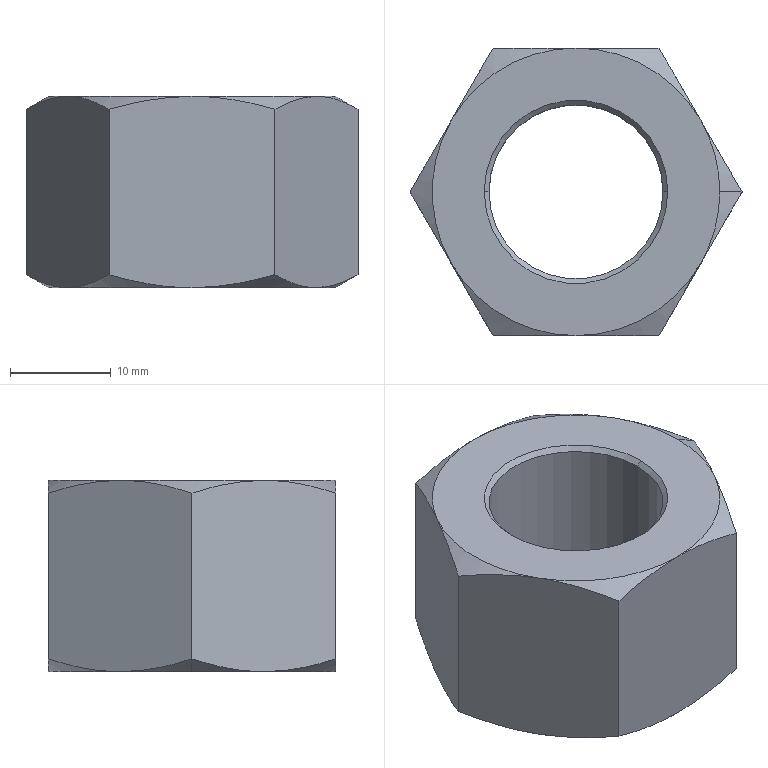Part | SolidWorks | 1 solid | 28 faces | box 33 x 28.579 x 19 mm | volume 8913 mm3 | cone 18 | plane 8 | cylinder 2 | commonest cylinder face diameters 17.294 x2
STEP:
#1=CARTESIAN_POINT('',(-8.647,0.,18.525));
#2=VERTEX_POINT('',#1);
#3=CARTESIAN_POINT('',(8.647,0.,18.525));
#4=VERTEX_POINT('',#3);
#5=CARTESIAN_POINT('',(0.,0.,18.525));
#6=DIRECTION('',(0.,0.,1.));
#7=DIRECTION('',(1.,0.,0.));
#8=AXIS2_PLACEMENT_3D('',#5,#6,#7);
#9=CIRCLE('',#8,8.647);
#10=EDGE_CURVE('',#2,#4,#9,.T.);
#11=ORIENTED_EDGE('',*,*,#10,.F.);
#12=CARTESIAN_POINT('',(-9.122,0.,19.));
#13=VERTEX_POINT('',#12);
#14=CARTESIAN_POINT('',(-8.647,0.,18.525));
#15=DIRECTION('',(-0.7071,0.,0.7071));
#16=VECTOR('',#15,1000.);
#17=LINE('',#14,#16);
#18=EDGE_CURVE('',#2,#13,#17,.T.);
#19=ORIENTED_EDGE('',*,*,#18,.T.);
#20=CARTESIAN_POINT('',(9.122,0.,19.));
#21=VERTEX_POINT('',#20);
#22=CARTESIAN_POINT('',(0.,0.,19.));
#23=DIRECTION('',(0.,0.,-1.));
#24=DIRECTION('',(1.,0.,0.));
#25=AXIS2_PLACEMENT_3D('',#22,#23,#24);
#26=CIRCLE('',#25,9.122);
#27=EDGE_CURVE('',#21,#13,#26,.T.);
#28=ORIENTED_EDGE('',*,*,#27,.F.);
#29=CARTESIAN_POINT('',(8.647,0.,18.525));
#30=DIRECTION('',(0.7071,0.,0.7071));
#31=VECTOR('',#30,1000.);
#32=LINE('',#29,#31);
#33=EDGE_CURVE('',#4,#21,#32,.T.);
#34=ORIENTED_EDGE('',*,*,#33,.F.);
#35=EDGE_LOOP('',(#11,#19,#28,#34));
#36=FACE_OUTER_BOUND('',#35,.T.);
#37=CARTESIAN_POINT('',(0.,0.,18.525));
#38=DIRECTION('',(0.,0.,1.));
#39=DIRECTION('',(1.,0.,0.));
#40=AXIS2_PLACEMENT_3D('',#37,#38,#39);
#41=CONICAL_SURFACE('',#40,8.647,0.7854);
#42=ADVANCED_FACE('',(#36),#41,.F.);
#43=CARTESIAN_POINT('',(8.647,0.,0.475));
#44=VERTEX_POINT('',#43);
#45=CARTESIAN_POINT('',(-8.647,0.,0.475));
#46=VERTEX_POINT('',#45);
#47=CARTESIAN_POINT('',(0.,0.,0.475));
#48=DIRECTION('',(0.,0.,-1.));
#49=DIRECTION('',(1.,0.,0.));
#50=AXIS2_PLACEMENT_3D('',#47,#48,#49);
#51=CIRCLE('',#50,8.647);
#52=EDGE_CURVE('',#44,#46,#51,.T.);
#53=ORIENTED_EDGE('',*,*,#52,.F.);
#54=CARTESIAN_POINT('',(9.122,0.,0.));
#55=VERTEX_POINT('',#54);
#56=CARTESIAN_POINT('',(9.122,0.,0.));
#57=DIRECTION('',(0.7071,0.,-0.7071));
#58=VECTOR('',#57,1000.);
#59=LINE('',#56,#58);
#60=EDGE_CURVE('',#44,#55,#59,.T.);
#61=ORIENTED_EDGE('',*,*,#60,.T.);
#62=CARTESIAN_POINT('',(-9.122,0.,0.));
#63=VERTEX_POINT('',#62);
#64=CARTESIAN_POINT('',(0.,0.,0.));
#65=DIRECTION('',(0.,0.,1.));
#66=DIRECTION('',(1.,0.,0.));
#67=AXIS2_PLACEMENT_3D('',#64,#65,#66);
#68=CIRCLE('',#67,9.122);
#69=EDGE_CURVE('',#63,#55,#68,.T.);
#70=ORIENTED_EDGE('',*,*,#69,.F.);
#71=CARTESIAN_POINT('',(-9.122,0.,0.));
#72=DIRECTION('',(-0.7071,0.,-0.7071));
#73=VECTOR('',#72,1000.);
#74=LINE('',#71,#73);
#75=EDGE_CURVE('',#46,#63,#74,.T.);
#76=ORIENTED_EDGE('',*,*,#75,.F.);
#77=EDGE_LOOP('',(#53,#61,#70,#76));
#78=FACE_OUTER_BOUND('',#77,.T.);
#79=CARTESIAN_POINT('',(0.,0.,0.));
#80=DIRECTION('',(0.,0.,-1.));
#81=DIRECTION('',(-1.,0.,0.));
#82=AXIS2_PLACEMENT_3D('',#79,#80,#81);
#83=CONICAL_SURFACE('',#82,9.122,0.7854);
#84=ADVANCED_FACE('',(#78),#83,.F.);
#85=CARTESIAN_POINT('',(14.289,0.,19.));
#86=VERTEX_POINT('',#85);
#87=CARTESIAN_POINT('',(12.375,7.145,19.));
#88=VERTEX_POINT('',#87);
#89=CARTESIAN_POINT('',(0.,0.,19.));
#90=DIRECTION('',(0.,0.,1.));
#91=DIRECTION('',(1.,0.,0.));
#92=AXIS2_PLACEMENT_3D('',#89,#90,#91);
#93=CIRCLE('',#92,14.289);
#94=EDGE_CURVE('',#86,#88,#93,.T.);
#95=ORIENTED_EDGE('',*,*,#94,.F.);
#96=CARTESIAN_POINT('',(16.5,0.,17.724));
#97=VERTEX_POINT('',#96);
#98=CARTESIAN_POINT('',(14.289,0.,19.));
#99=DIRECTION('',(0.866,0.,-0.5));
#100=VECTOR('',#99,1000.);
#101=LINE('',#98,#100);
#102=EDGE_CURVE('',#86,#97,#101,.T.);
#103=ORIENTED_EDGE('',*,*,#102,.T.);
#104=CARTESIAN_POINT('',(16.5,0.,17.724));
#105=CARTESIAN_POINT('',(15.825,1.169,18.113));
#106=CARTESIAN_POINT('',(15.145,2.346,18.434));
#107=CARTESIAN_POINT('',(13.772,4.725,18.878));
#108=CARTESIAN_POINT('',(13.078,5.927,19.));
#109=CARTESIAN_POINT('',(12.375,7.145,19.));
#110=B_SPLINE_CURVE_WITH_KNOTS('',3,(#104,#105,#106,#107,#108,#109),.UNSPECIFIED.,.F.,.F.,(4,2,4),(0.000000238,0.004174,0.008348),.UNSPECIFIED.);
#111=EDGE_CURVE('',#97,#88,#110,.T.);
#112=ORIENTED_EDGE('',*,*,#111,.T.);
#113=EDGE_LOOP('',(#95,#103,#112));
#114=FACE_OUTER_BOUND('',#113,.T.);
#115=CARTESIAN_POINT('',(0.,0.,19.));
#116=DIRECTION('',(0.,0.,-1.));
#117=DIRECTION('',(1.,0.,0.));
#118=AXIS2_PLACEMENT_3D('',#115,#116,#117);
#119=CONICAL_SURFACE('',#118,14.289,1.047);
#120=ADVANCED_FACE('',(#114),#119,.T.);
#121=CARTESIAN_POINT('',(-14.289,0.,0.));
#122=VERTEX_POINT('',#121);
#123=CARTESIAN_POINT('',(-12.375,7.145,0.));
#124=VERTEX_POINT('',#123);
#125=CARTESIAN_POINT('',(0.,0.,0.));
#126=DIRECTION('',(0.,0.,-1.));
#127=DIRECTION('',(-1.,0.,0.));
#128=AXIS2_PLACEMENT_3D('',#125,#126,#127);
#129=CIRCLE('',#128,14.289);
#130=EDGE_CURVE('',#122,#124,#129,.T.);
#131=ORIENTED_EDGE('',*,*,#130,.F.);
#132=CARTESIAN_POINT('',(-16.5,0.,1.276));
#133=VERTEX_POINT('',#132);
#134=CARTESIAN_POINT('',(-14.289,0.,0.));
#135=DIRECTION('',(-0.866,0.,0.5));
#136=VECTOR('',#135,1000.);
#137=LINE('',#134,#136);
#138=EDGE_CURVE('',#122,#133,#137,.T.);
#139=ORIENTED_EDGE('',*,*,#138,.T.);
#140=CARTESIAN_POINT('',(-16.5,0.,1.276));
#141=CARTESIAN_POINT('',(-15.825,1.169,0.8867));
#142=CARTESIAN_POINT('',(-15.145,2.346,0.5657));
#143=CARTESIAN_POINT('',(-13.772,4.725,0.1216));
#144=CARTESIAN_POINT('',(-13.078,5.927,0.));
#145=CARTESIAN_POINT('',(-12.375,7.145,0.));
#146=B_SPLINE_CURVE_WITH_KNOTS('',3,(#140,#141,#142,#143,#144,#145),.UNSPECIFIED.,.F.,.F.,(4,2,4),(0.000000238,0.004174,0.008348),.UNSPECIFIED.);
#147=EDGE_CURVE('',#133,#124,#146,.T.);
#148=ORIENTED_EDGE('',*,*,#147,.T.);
#149=EDGE_LOOP('',(#131,#139,#148));
#150=FACE_OUTER_BOUND('',#149,.T.);
#151=CARTESIAN_POINT('',(0.,0.,0.));
#152=DIRECTION('',(0.,0.,1.));
#153=DIRECTION('',(-1.,0.,0.));
#154=AXIS2_PLACEMENT_3D('',#151,#152,#153);
#155=CONICAL_SURFACE('',#154,14.289,1.047);
#156=ADVANCED_FACE('',(#150),#155,.T.);
#157=ORIENTED_EDGE('',*,*,#10,.T.);
#158=CARTESIAN_POINT('',(8.647,0.,19.));
#159=DIRECTION('',(0.,0.,-1.));
#160=VECTOR('',#159,1000.);
#161=LINE('',#158,#160);
#162=EDGE_CURVE('',#4,#44,#161,.T.);
#163=ORIENTED_EDGE('',*,*,#162,.T.);
#164=ORIENTED_EDGE('',*,*,#52,.T.);
#165=CARTESIAN_POINT('',(-8.647,0.,19.));
#166=DIRECTION('',(0.,0.,-1.));
#167=VECTOR('',#166,1000.);
#168=LINE('',#165,#167);
#169=EDGE_CURVE('',#2,#46,#168,.T.);
#170=ORIENTED_EDGE('',*,*,#169,.F.);
#171=EDGE_LOOP('',(#157,#163,#164,#170));
#172=FACE_OUTER_BOUND('',#171,.T.);
#173=CARTESIAN_POINT('',(0.,0.,19.));
#174=DIRECTION('',(0.,0.,-1.));
#175=DIRECTION('',(-1.,0.,0.));
#176=AXIS2_PLACEMENT_3D('',#173,#174,#175);
#177=CYLINDRICAL_SURFACE('',#176,8.647);
#178=ADVANCED_FACE('',(#172),#177,.F.);
#179=ORIENTED_EDGE('',*,*,#111,.F.);
#180=CARTESIAN_POINT('',(16.5,0.,1.276));
#181=VERTEX_POINT('',#180);
#182=CARTESIAN_POINT('',(16.5,0.,19.));
#183=DIRECTION('',(0.,0.,-1.));
#184=VECTOR('',#183,1000.);
#185=LINE('',#182,#184);
#186=EDGE_CURVE('',#97,#181,#185,.T.);
#187=ORIENTED_EDGE('',*,*,#186,.T.);
#188=CARTESIAN_POINT('',(12.375,7.145,0.));
#189=VERTEX_POINT('',#188);
#190=CARTESIAN_POINT('',(12.375,7.145,0.));
#191=CARTESIAN_POINT('',(12.725,6.538,0.));
#192=CARTESIAN_POINT('',(13.077,5.929,0.03017));
#193=CARTESIAN_POINT('',(13.772,4.724,0.1469));
#194=CARTESIAN_POINT('',(14.118,4.126,0.2334));
#195=CARTESIAN_POINT('',(15.148,2.341,0.5668));
#196=CARTESIAN_POINT('',(15.827,1.166,0.8877));
#197=CARTESIAN_POINT('',(16.5,0.,1.276));
#198=B_SPLINE_CURVE_WITH_KNOTS('',3,(#190,#191,#192,#193,#194,#195,#196,#197),.UNSPECIFIED.,.F.,.F.,(4,2,2,4),(0.008348,0.01043,0.01251,0.01666),.UNSPECIFIED.);
#199=EDGE_CURVE('',#189,#181,#198,.T.);
#200=ORIENTED_EDGE('',*,*,#199,.F.);
#201=CARTESIAN_POINT('',(8.25,14.289,1.276));
#202=VERTEX_POINT('',#201);
#203=CARTESIAN_POINT('',(8.25,14.289,1.276));
#204=CARTESIAN_POINT('',(8.925,13.121,0.8867));
#205=CARTESIAN_POINT('',(9.605,11.943,0.5657));
#206=CARTESIAN_POINT('',(10.978,9.564,0.1216));
#207=CARTESIAN_POINT('',(11.672,8.362,0.));
#208=CARTESIAN_POINT('',(12.375,7.145,0.));
#209=B_SPLINE_CURVE_WITH_KNOTS('',3,(#203,#204,#205,#206,#207,#208),.UNSPECIFIED.,.F.,.F.,(4,2,4),(0.000000238,0.004174,0.008348),.UNSPECIFIED.);
#210=EDGE_CURVE('',#202,#189,#209,.T.);
#211=ORIENTED_EDGE('',*,*,#210,.F.);
#212=CARTESIAN_POINT('',(8.25,14.289,17.724));
#213=VERTEX_POINT('',#212);
#214=CARTESIAN_POINT('',(8.25,14.289,19.));
#215=DIRECTION('',(0.,0.,-1.));
#216=VECTOR('',#215,1000.);
#217=LINE('',#214,#216);
#218=EDGE_CURVE('',#213,#202,#217,.T.);
#219=ORIENTED_EDGE('',*,*,#218,.F.);
#220=CARTESIAN_POINT('',(12.375,7.145,19.));
#221=CARTESIAN_POINT('',(12.025,7.751,19.));
#222=CARTESIAN_POINT('',(11.673,8.36,18.97));
#223=CARTESIAN_POINT('',(10.978,9.565,18.853));
#224=CARTESIAN_POINT('',(10.632,10.163,18.767));
#225=CARTESIAN_POINT('',(9.602,11.948,18.433));
#226=CARTESIAN_POINT('',(8.923,13.124,18.112));
#227=CARTESIAN_POINT('',(8.25,14.289,17.724));
#228=B_SPLINE_CURVE_WITH_KNOTS('',3,(#220,#221,#222,#223,#224,#225,#226,#227),.UNSPECIFIED.,.F.,.F.,(4,2,2,4),(0.008348,0.01043,0.01251,0.01666),.UNSPECIFIED.);
#229=EDGE_CURVE('',#88,#213,#228,.T.);
#230=ORIENTED_EDGE('',*,*,#229,.F.);
#231=EDGE_LOOP('',(#179,#187,#200,#211,#219,#230));
#232=FACE_OUTER_BOUND('',#231,.T.);
#233=CARTESIAN_POINT('',(16.5,0.,19.));
#234=DIRECTION('',(-0.866,-0.5,0.));
#235=DIRECTION('',(0.5,-0.866,0.));
#236=AXIS2_PLACEMENT_3D('',#233,#234,#235);
#237=PLANE('',#236);
#238=ADVANCED_FACE('',(#232),#237,.F.);
#239=CARTESIAN_POINT('',(0.,14.289,19.));
#240=VERTEX_POINT('',#239);
#241=CARTESIAN_POINT('',(8.25,14.289,17.724));
#242=CARTESIAN_POINT('',(6.916,14.289,18.109));
#243=CARTESIAN_POINT('',(5.564,14.289,18.429));
#244=CARTESIAN_POINT('',(3.499,14.289,18.765));
#245=CARTESIAN_POINT('',(2.804,14.289,18.852));
#246=CARTESIAN_POINT('',(1.4,14.289,18.97));
#247=CARTESIAN_POINT('',(0.6982,14.289,19.));
#248=CARTESIAN_POINT('',(0.,14.289,19.));
#249=B_SPLINE_CURVE_WITH_KNOTS('',3,(#241,#242,#243,#244,#245,#246,#247,#248),.UNSPECIFIED.,.F.,.F.,(4,2,2,4),(0.04793,0.0521,0.05419,0.05628),.UNSPECIFIED.);
#250=EDGE_CURVE('',#213,#240,#249,.T.);
#251=ORIENTED_EDGE('',*,*,#250,.F.);
#252=ORIENTED_EDGE('',*,*,#218,.T.);
#253=CARTESIAN_POINT('',(0.,14.289,0.));
#254=VERTEX_POINT('',#253);
#255=CARTESIAN_POINT('',(0.,14.289,0.));
#256=CARTESIAN_POINT('',(0.6982,14.289,0.));
#257=CARTESIAN_POINT('',(1.4,14.289,0.02979));
#258=CARTESIAN_POINT('',(2.804,14.289,0.1478));
#259=CARTESIAN_POINT('',(3.499,14.289,0.2352));
#260=CARTESIAN_POINT('',(5.564,14.289,0.5705));
#261=CARTESIAN_POINT('',(6.916,14.289,0.8911));
#262=CARTESIAN_POINT('',(8.25,14.289,1.276));
#263=B_SPLINE_CURVE_WITH_KNOTS('',3,(#255,#256,#257,#258,#259,#260,#261,#262),.UNSPECIFIED.,.F.,.F.,(4,2,2,4),(0.02351,0.0256,0.02769,0.03187),.UNSPECIFIED.);
#264=EDGE_CURVE('',#254,#202,#263,.T.);
#265=ORIENTED_EDGE('',*,*,#264,.F.);
#266=CARTESIAN_POINT('',(-8.25,14.289,1.276));
#267=VERTEX_POINT('',#266);
#268=CARTESIAN_POINT('',(-8.25,14.289,1.276));
#269=CARTESIAN_POINT('',(-6.907,14.289,0.8886));
#270=CARTESIAN_POINT('',(-5.533,14.289,0.564));
#271=CARTESIAN_POINT('',(-2.781,14.289,0.12));
#272=CARTESIAN_POINT('',(-1.395,14.289,0.));
#273=CARTESIAN_POINT('',(0.,14.289,0.));
#274=B_SPLINE_CURVE_WITH_KNOTS('',3,(#268,#269,#270,#271,#272,#273),.UNSPECIFIED.,.F.,.F.,(4,2,4),(0.01516,0.01934,0.02351),.UNSPECIFIED.);
#275=EDGE_CURVE('',#267,#254,#274,.T.);
#276=ORIENTED_EDGE('',*,*,#275,.F.);
#277=CARTESIAN_POINT('',(-8.25,14.289,17.724));
#278=VERTEX_POINT('',#277);
#279=CARTESIAN_POINT('',(-8.25,14.289,19.));
#280=DIRECTION('',(0.,0.,-1.));
#281=VECTOR('',#280,1000.);
#282=LINE('',#279,#281);
#283=EDGE_CURVE('',#278,#267,#282,.T.);
#284=ORIENTED_EDGE('',*,*,#283,.F.);
#285=CARTESIAN_POINT('',(0.,14.289,19.));
#286=CARTESIAN_POINT('',(-1.395,14.289,19.));
#287=CARTESIAN_POINT('',(-2.781,14.289,18.88));
#288=CARTESIAN_POINT('',(-5.533,14.289,18.436));
#289=CARTESIAN_POINT('',(-6.907,14.289,18.111));
#290=CARTESIAN_POINT('',(-8.25,14.289,17.724));
#291=B_SPLINE_CURVE_WITH_KNOTS('',3,(#285,#286,#287,#288,#289,#290),.UNSPECIFIED.,.F.,.F.,(4,2,4),(0.05628,0.06045,0.06463),.UNSPECIFIED.);
#292=EDGE_CURVE('',#240,#278,#291,.T.);
#293=ORIENTED_EDGE('',*,*,#292,.F.);
#294=EDGE_LOOP('',(#251,#252,#265,#276,#284,#293));
#295=FACE_OUTER_BOUND('',#294,.T.);
#296=CARTESIAN_POINT('',(8.25,14.289,19.));
#297=DIRECTION('',(0.,-1.,0.));
#298=DIRECTION('',(1.,0.,0.));
#299=AXIS2_PLACEMENT_3D('',#296,#297,#298);
#300=PLANE('',#299);
#301=ADVANCED_FACE('',(#295),#300,.F.);
#302=CARTESIAN_POINT('',(-12.375,7.145,19.));
#303=VERTEX_POINT('',#302);
#304=CARTESIAN_POINT('',(-8.25,14.289,17.724));
#305=CARTESIAN_POINT('',(-8.925,13.121,18.113));
#306=CARTESIAN_POINT('',(-9.605,11.943,18.434));
#307=CARTESIAN_POINT('',(-10.978,9.564,18.878));
#308=CARTESIAN_POINT('',(-11.672,8.362,19.));
#309=CARTESIAN_POINT('',(-12.375,7.145,19.));
#310=B_SPLINE_CURVE_WITH_KNOTS('',3,(#304,#305,#306,#307,#308,#309),.UNSPECIFIED.,.F.,.F.,(4,2,4),(0.000000238,0.004174,0.008348),.UNSPECIFIED.);
#311=EDGE_CURVE('',#278,#303,#310,.T.);
#312=ORIENTED_EDGE('',*,*,#311,.F.);
#313=ORIENTED_EDGE('',*,*,#283,.T.);
#314=CARTESIAN_POINT('',(-12.375,7.145,0.));
#315=CARTESIAN_POINT('',(-12.025,7.751,0.));
#316=CARTESIAN_POINT('',(-11.673,8.36,0.03017));
#317=CARTESIAN_POINT('',(-10.978,9.565,0.1469));
#318=CARTESIAN_POINT('',(-10.632,10.163,0.2334));
#319=CARTESIAN_POINT('',(-9.602,11.948,0.5668));
#320=CARTESIAN_POINT('',(-8.923,13.124,0.8877));
#321=CARTESIAN_POINT('',(-8.25,14.289,1.276));
#322=B_SPLINE_CURVE_WITH_KNOTS('',3,(#314,#315,#316,#317,#318,#319,#320,#321),.UNSPECIFIED.,.F.,.F.,(4,2,2,4),(0.008348,0.01043,0.01251,0.01666),.UNSPECIFIED.);
#323=EDGE_CURVE('',#124,#267,#322,.T.);
#324=ORIENTED_EDGE('',*,*,#323,.F.);
#325=ORIENTED_EDGE('',*,*,#147,.F.);
#326=CARTESIAN_POINT('',(-16.5,0.,17.724));
#327=VERTEX_POINT('',#326);
#328=CARTESIAN_POINT('',(-16.5,0.,19.));
#329=DIRECTION('',(0.,0.,-1.));
#330=VECTOR('',#329,1000.);
#331=LINE('',#328,#330);
#332=EDGE_CURVE('',#327,#133,#331,.T.);
#333=ORIENTED_EDGE('',*,*,#332,.F.);
#334=CARTESIAN_POINT('',(-12.375,7.145,19.));
#335=CARTESIAN_POINT('',(-12.725,6.538,19.));
#336=CARTESIAN_POINT('',(-13.077,5.929,18.97));
#337=CARTESIAN_POINT('',(-13.772,4.724,18.853));
#338=CARTESIAN_POINT('',(-14.118,4.126,18.767));
#339=CARTESIAN_POINT('',(-15.148,2.341,18.433));
#340=CARTESIAN_POINT('',(-15.827,1.166,18.112));
#341=CARTESIAN_POINT('',(-16.5,0.,17.724));
#342=B_SPLINE_CURVE_WITH_KNOTS('',3,(#334,#335,#336,#337,#338,#339,#340,#341),.UNSPECIFIED.,.F.,.F.,(4,2,2,4),(0.008348,0.01043,0.01251,0.01666),.UNSPECIFIED.);
#343=EDGE_CURVE('',#303,#327,#342,.T.);
#344=ORIENTED_EDGE('',*,*,#343,.F.);
#345=EDGE_LOOP('',(#312,#313,#324,#325,#333,#344));
#346=FACE_OUTER_BOUND('',#345,.T.);
#347=CARTESIAN_POINT('',(-8.25,14.289,19.));
#348=DIRECTION('',(0.866,-0.5,0.));
#349=DIRECTION('',(0.5,0.866,0.));
#350=AXIS2_PLACEMENT_3D('',#347,#348,#349);
#351=PLANE('',#350);
#352=ADVANCED_FACE('',(#346),#351,.F.);
#353=CARTESIAN_POINT('',(-12.375,-7.145,19.));
#354=VERTEX_POINT('',#353);
#355=CARTESIAN_POINT('',(-16.5,0.,17.724));
#356=CARTESIAN_POINT('',(-15.825,-1.169,18.113));
#357=CARTESIAN_POINT('',(-15.145,-2.346,18.434));
#358=CARTESIAN_POINT('',(-13.772,-4.725,18.878));
#359=CARTESIAN_POINT('',(-13.078,-5.927,19.));
#360=CARTESIAN_POINT('',(-12.375,-7.145,19.));
#361=B_SPLINE_CURVE_WITH_KNOTS('',3,(#355,#356,#357,#358,#359,#360),.UNSPECIFIED.,.F.,.F.,(4,2,4),(0.000000238,0.004174,0.008348),.UNSPECIFIED.);
#362=EDGE_CURVE('',#327,#354,#361,.T.);
#363=ORIENTED_EDGE('',*,*,#362,.F.);
#364=ORIENTED_EDGE('',*,*,#332,.T.);
#365=CARTESIAN_POINT('',(-12.375,-7.145,0.));
#366=VERTEX_POINT('',#365);
#367=CARTESIAN_POINT('',(-12.375,-7.145,0.));
#368=CARTESIAN_POINT('',(-12.725,-6.538,0.));
#369=CARTESIAN_POINT('',(-13.077,-5.929,0.03017));
#370=CARTESIAN_POINT('',(-13.772,-4.724,0.1469));
#371=CARTESIAN_POINT('',(-14.118,-4.126,0.2334));
#372=CARTESIAN_POINT('',(-15.148,-2.341,0.5668));
#373=CARTESIAN_POINT('',(-15.827,-1.166,0.8877));
#374=CARTESIAN_POINT('',(-16.5,0.,1.276));
#375=B_SPLINE_CURVE_WITH_KNOTS('',3,(#367,#368,#369,#370,#371,#372,#373,#374),.UNSPECIFIED.,.F.,.F.,(4,2,2,4),(0.008348,0.01043,0.01251,0.01666),.UNSPECIFIED.);
#376=EDGE_CURVE('',#366,#133,#375,.T.);
#377=ORIENTED_EDGE('',*,*,#376,.F.);
#378=CARTESIAN_POINT('',(-8.25,-14.289,1.276));
#379=VERTEX_POINT('',#378);
#380=CARTESIAN_POINT('',(-8.25,-14.289,1.276));
#381=CARTESIAN_POINT('',(-8.925,-13.121,0.8867));
#382=CARTESIAN_POINT('',(-9.605,-11.943,0.5657));
#383=CARTESIAN_POINT('',(-10.978,-9.564,0.1216));
#384=CARTESIAN_POINT('',(-11.672,-8.362,0.));
#385=CARTESIAN_POINT('',(-12.375,-7.145,0.));
#386=B_SPLINE_CURVE_WITH_KNOTS('',3,(#380,#381,#382,#383,#384,#385),.UNSPECIFIED.,.F.,.F.,(4,2,4),(0.000000238,0.004174,0.008348),.UNSPECIFIED.);
#387=EDGE_CURVE('',#379,#366,#386,.T.);
#388=ORIENTED_EDGE('',*,*,#387,.F.);
#389=CARTESIAN_POINT('',(-8.25,-14.289,17.724));
#390=VERTEX_POINT('',#389);
#391=CARTESIAN_POINT('',(-8.25,-14.289,19.));
#392=DIRECTION('',(0.,0.,-1.));
#393=VECTOR('',#392,1000.);
#394=LINE('',#391,#393);
#395=EDGE_CURVE('',#390,#379,#394,.T.);
#396=ORIENTED_EDGE('',*,*,#395,.F.);
#397=CARTESIAN_POINT('',(-12.375,-7.145,19.));
#398=CARTESIAN_POINT('',(-12.025,-7.751,19.));
#399=CARTESIAN_POINT('',(-11.673,-8.36,18.97));
#400=CARTESIAN_POINT('',(-10.978,-9.565,18.853));
#401=CARTESIAN_POINT('',(-10.632,-10.163,18.767));
#402=CARTESIAN_POINT('',(-9.602,-11.948,18.433));
#403=CARTESIAN_POINT('',(-8.923,-13.124,18.112));
#404=CARTESIAN_POINT('',(-8.25,-14.289,17.724));
#405=B_SPLINE_CURVE_WITH_KNOTS('',3,(#397,#398,#399,#400,#401,#402,#403,#404),.UNSPECIFIED.,.F.,.F.,(4,2,2,4),(0.008348,0.01043,0.01251,0.01666),.UNSPECIFIED.);
#406=EDGE_CURVE('',#354,#390,#405,.T.);
#407=ORIENTED_EDGE('',*,*,#406,.F.);
#408=EDGE_LOOP('',(#363,#364,#377,#388,#396,#407));
#409=FACE_OUTER_BOUND('',#408,.T.);
#410=CARTESIAN_POINT('',(-16.5,0.,19.));
#411=DIRECTION('',(0.866,0.5,0.));
#412=DIRECTION('',(-0.5,0.866,0.));
#413=AXIS2_PLACEMENT_3D('',#410,#411,#412);
#414=PLANE('',#413);
#415=ADVANCED_FACE('',(#409),#414,.F.);
#416=CARTESIAN_POINT('',(0.,-14.289,19.));
#417=VERTEX_POINT('',#416);
#418=CARTESIAN_POINT('',(-8.25,-14.289,17.724));
#419=CARTESIAN_POINT('',(-6.907,-14.289,18.111));
#420=CARTESIAN_POINT('',(-5.533,-14.289,18.436));
#421=CARTESIAN_POINT('',(-2.781,-14.289,18.88));
#422=CARTESIAN_POINT('',(-1.395,-14.289,19.));
#423=CARTESIAN_POINT('',(0.,-14.289,19.));
#424=B_SPLINE_CURVE_WITH_KNOTS('',3,(#418,#419,#420,#421,#422,#423),.UNSPECIFIED.,.F.,.F.,(4,2,4),(0.01516,0.01934,0.02351),.UNSPECIFIED.);
#425=EDGE_CURVE('',#390,#417,#424,.T.);
#426=ORIENTED_EDGE('',*,*,#425,.F.);
#427=ORIENTED_EDGE('',*,*,#395,.T.);
#428=CARTESIAN_POINT('',(0.,-14.289,0.));
#429=VERTEX_POINT('',#428);
#430=CARTESIAN_POINT('',(0.,-14.289,0.));
#431=CARTESIAN_POINT('',(-1.395,-14.289,0.));
#432=CARTESIAN_POINT('',(-2.781,-14.289,0.12));
#433=CARTESIAN_POINT('',(-5.533,-14.289,0.564));
#434=CARTESIAN_POINT('',(-6.907,-14.289,0.8886));
#435=CARTESIAN_POINT('',(-8.25,-14.289,1.276));
#436=B_SPLINE_CURVE_WITH_KNOTS('',3,(#430,#431,#432,#433,#434,#435),.UNSPECIFIED.,.F.,.F.,(4,2,4),(0.05628,0.06045,0.06463),.UNSPECIFIED.);
#437=EDGE_CURVE('',#429,#379,#436,.T.);
#438=ORIENTED_EDGE('',*,*,#437,.F.);
#439=CARTESIAN_POINT('',(8.25,-14.289,1.276));
#440=VERTEX_POINT('',#439);
#441=CARTESIAN_POINT('',(8.25,-14.289,1.276));
#442=CARTESIAN_POINT('',(6.916,-14.289,0.8911));
#443=CARTESIAN_POINT('',(5.564,-14.289,0.5705));
#444=CARTESIAN_POINT('',(3.499,-14.289,0.2352));
#445=CARTESIAN_POINT('',(2.804,-14.289,0.1478));
#446=CARTESIAN_POINT('',(1.4,-14.289,0.02979));
#447=CARTESIAN_POINT('',(0.6982,-14.289,0.));
#448=CARTESIAN_POINT('',(0.,-14.289,0.));
#449=B_SPLINE_CURVE_WITH_KNOTS('',3,(#441,#442,#443,#444,#445,#446,#447,#448),.UNSPECIFIED.,.F.,.F.,(4,2,2,4),(0.04793,0.0521,0.05419,0.05628),.UNSPECIFIED.);
#450=EDGE_CURVE('',#440,#429,#449,.T.);
#451=ORIENTED_EDGE('',*,*,#450,.F.);
#452=CARTESIAN_POINT('',(8.25,-14.289,17.724));
#453=VERTEX_POINT('',#452);
#454=CARTESIAN_POINT('',(8.25,-14.289,19.));
#455=DIRECTION('',(0.,0.,-1.));
#456=VECTOR('',#455,1000.);
#457=LINE('',#454,#456);
#458=EDGE_CURVE('',#453,#440,#457,.T.);
#459=ORIENTED_EDGE('',*,*,#458,.F.);
#460=CARTESIAN_POINT('',(0.,-14.289,19.));
#461=CARTESIAN_POINT('',(0.6982,-14.289,19.));
#462=CARTESIAN_POINT('',(1.4,-14.289,18.97));
#463=CARTESIAN_POINT('',(2.804,-14.289,18.852));
#464=CARTESIAN_POINT('',(3.499,-14.289,18.765));
#465=CARTESIAN_POINT('',(5.564,-14.289,18.429));
#466=CARTESIAN_POINT('',(6.916,-14.289,18.109));
#467=CARTESIAN_POINT('',(8.25,-14.289,17.724));
#468=B_SPLINE_CURVE_WITH_KNOTS('',3,(#460,#461,#462,#463,#464,#465,#466,#467),.UNSPECIFIED.,.F.,.F.,(4,2,2,4),(0.02351,0.0256,0.02769,0.03187),.UNSPECIFIED.);
#469=EDGE_CURVE('',#417,#453,#468,.T.);
#470=ORIENTED_EDGE('',*,*,#469,.F.);
#471=EDGE_LOOP('',(#426,#427,#438,#451,#459,#470));
#472=FACE_OUTER_BOUND('',#471,.T.);
#473=CARTESIAN_POINT('',(-8.25,-14.289,19.));
#474=DIRECTION('',(0.,1.,0.));
#475=DIRECTION('',(-1.,0.,0.));
#476=AXIS2_PLACEMENT_3D('',#473,#474,#475);
#477=PLANE('',#476);
#478=ADVANCED_FACE('',(#472),#477,.F.);
#479=CARTESIAN_POINT('',(12.375,-7.145,19.));
#480=VERTEX_POINT('',#479);
#481=CARTESIAN_POINT('',(8.25,-14.289,17.724));
#482=CARTESIAN_POINT('',(8.925,-13.121,18.113));
#483=CARTESIAN_POINT('',(9.605,-11.943,18.434));
#484=CARTESIAN_POINT('',(10.978,-9.564,18.878));
#485=CARTESIAN_POINT('',(11.672,-8.362,19.));
#486=CARTESIAN_POINT('',(12.375,-7.145,19.));
#487=B_SPLINE_CURVE_WITH_KNOTS('',3,(#481,#482,#483,#484,#485,#486),.UNSPECIFIED.,.F.,.F.,(4,2,4),(0.000000238,0.004174,0.008348),.UNSPECIFIED.);
#488=EDGE_CURVE('',#453,#480,#487,.T.);
#489=ORIENTED_EDGE('',*,*,#488,.F.);
#490=ORIENTED_EDGE('',*,*,#458,.T.);
#491=CARTESIAN_POINT('',(12.375,-7.145,0.));
#492=VERTEX_POINT('',#491);
#493=CARTESIAN_POINT('',(12.375,-7.145,0.));
#494=CARTESIAN_POINT('',(12.025,-7.751,0.));
#495=CARTESIAN_POINT('',(11.673,-8.36,0.03017));
#496=CARTESIAN_POINT('',(10.978,-9.565,0.1469));
#497=CARTESIAN_POINT('',(10.632,-10.163,0.2334));
#498=CARTESIAN_POINT('',(9.602,-11.948,0.5668));
#499=CARTESIAN_POINT('',(8.923,-13.124,0.8877));
#500=CARTESIAN_POINT('',(8.25,-14.289,1.276));
#501=B_SPLINE_CURVE_WITH_KNOTS('',3,(#493,#494,#495,#496,#497,#498,#499,#500),.UNSPECIFIED.,.F.,.F.,(4,2,2,4),(0.008348,0.01043,0.01251,0.01666),.UNSPECIFIED.);
#502=EDGE_CURVE('',#492,#440,#501,.T.);
#503=ORIENTED_EDGE('',*,*,#502,.F.);
#504=CARTESIAN_POINT('',(16.5,0.,1.276));
#505=CARTESIAN_POINT('',(15.825,-1.169,0.8867));
#506=CARTESIAN_POINT('',(15.145,-2.346,0.5657));
#507=CARTESIAN_POINT('',(13.772,-4.725,0.1216));
#508=CARTESIAN_POINT('',(13.078,-5.927,0.));
#509=CARTESIAN_POINT('',(12.375,-7.145,0.));
#510=B_SPLINE_CURVE_WITH_KNOTS('',3,(#504,#505,#506,#507,#508,#509),.UNSPECIFIED.,.F.,.F.,(4,2,4),(0.000000238,0.004174,0.008348),.UNSPECIFIED.);
#511=EDGE_CURVE('',#181,#492,#510,.T.);
#512=ORIENTED_EDGE('',*,*,#511,.F.);
#513=ORIENTED_EDGE('',*,*,#186,.F.);
#514=CARTESIAN_POINT('',(12.375,-7.145,19.));
#515=CARTESIAN_POINT('',(12.725,-6.538,19.));
#516=CARTESIAN_POINT('',(13.077,-5.929,18.97));
#517=CARTESIAN_POINT('',(13.772,-4.724,18.853));
#518=CARTESIAN_POINT('',(14.118,-4.126,18.767));
#519=CARTESIAN_POINT('',(15.148,-2.341,18.433));
#520=CARTESIAN_POINT('',(15.827,-1.166,18.112));
#521=CARTESIAN_POINT('',(16.5,0.,17.724));
#522=B_SPLINE_CURVE_WITH_KNOTS('',3,(#514,#515,#516,#517,#518,#519,#520,#521),.UNSPECIFIED.,.F.,.F.,(4,2,2,4),(0.008348,0.01043,0.01251,0.01666),.UNSPECIFIED.);
#523=EDGE_CURVE('',#480,#97,#522,.T.);
#524=ORIENTED_EDGE('',*,*,#523,.F.);
#525=EDGE_LOOP('',(#489,#490,#503,#512,#513,#524));
#526=FACE_OUTER_BOUND('',#525,.T.);
#527=CARTESIAN_POINT('',(8.25,-14.289,19.));
#528=DIRECTION('',(-0.866,0.5,0.));
#529=DIRECTION('',(-0.5,-0.866,0.));
#530=AXIS2_PLACEMENT_3D('',#527,#528,#529);
#531=PLANE('',#530);
#532=ADVANCED_FACE('',(#526),#531,.F.);
#533=ORIENTED_EDGE('',*,*,#27,.T.);
#534=CARTESIAN_POINT('',(0.,0.,19.));
#535=DIRECTION('',(0.,0.,-1.));
#536=DIRECTION('',(1.,0.,0.));
#537=AXIS2_PLACEMENT_3D('',#534,#535,#536);
#538=CIRCLE('',#537,9.122);
#539=EDGE_CURVE('',#13,#21,#538,.T.);
#540=ORIENTED_EDGE('',*,*,#539,.T.);
#541=EDGE_LOOP('',(#533,#540));
#542=FACE_BOUND('',#541,.T.);
#543=CARTESIAN_POINT('',(0.,0.,19.));
#544=DIRECTION('',(0.,0.,1.));
#545=DIRECTION('',(1.,0.,0.));
#546=AXIS2_PLACEMENT_3D('',#543,#544,#545);
#547=CIRCLE('',#546,14.289);
#548=EDGE_CURVE('',#480,#86,#547,.T.);
#549=ORIENTED_EDGE('',*,*,#548,.T.);
#550=ORIENTED_EDGE('',*,*,#94,.T.);
#551=CARTESIAN_POINT('',(0.,0.,19.));
#552=DIRECTION('',(0.,0.,1.));
#553=DIRECTION('',(1.,0.,0.));
#554=AXIS2_PLACEMENT_3D('',#551,#552,#553);
#555=CIRCLE('',#554,14.289);
#556=EDGE_CURVE('',#88,#240,#555,.T.);
#557=ORIENTED_EDGE('',*,*,#556,.T.);
#558=CARTESIAN_POINT('',(0.,0.,19.));
#559=DIRECTION('',(0.,0.,1.));
#560=DIRECTION('',(1.,0.,0.));
#561=AXIS2_PLACEMENT_3D('',#558,#559,#560);
#562=CIRCLE('',#561,14.289);
#563=EDGE_CURVE('',#240,#303,#562,.T.);
#564=ORIENTED_EDGE('',*,*,#563,.T.);
#565=CARTESIAN_POINT('',(0.,0.,19.));
#566=DIRECTION('',(0.,0.,1.));
#567=DIRECTION('',(1.,0.,0.));
#568=AXIS2_PLACEMENT_3D('',#565,#566,#567);
#569=CIRCLE('',#568,14.289);
#570=EDGE_CURVE('',#303,#354,#569,.T.);
#571=ORIENTED_EDGE('',*,*,#570,.T.);
#572=CARTESIAN_POINT('',(0.,0.,19.));
#573=DIRECTION('',(0.,0.,1.));
#574=DIRECTION('',(1.,0.,0.));
#575=AXIS2_PLACEMENT_3D('',#572,#573,#574);
#576=CIRCLE('',#575,14.289);
#577=EDGE_CURVE('',#354,#417,#576,.T.);
#578=ORIENTED_EDGE('',*,*,#577,.T.);
#579=CARTESIAN_POINT('',(0.,0.,19.));
#580=DIRECTION('',(0.,0.,1.));
#581=DIRECTION('',(1.,0.,0.));
#582=AXIS2_PLACEMENT_3D('',#579,#580,#581);
#583=CIRCLE('',#582,14.289);
#584=EDGE_CURVE('',#417,#480,#583,.T.);
#585=ORIENTED_EDGE('',*,*,#584,.T.);
#586=EDGE_LOOP('',(#549,#550,#557,#564,#571,#578,#585));
#587=FACE_OUTER_BOUND('',#586,.T.);
#588=CARTESIAN_POINT('',(0.,28.579,19.));
#589=DIRECTION('',(0.,0.,1.));
#590=DIRECTION('',(1.,0.,0.));
#591=AXIS2_PLACEMENT_3D('',#588,#589,#590);
#592=PLANE('',#591);
#593=ADVANCED_FACE('',(#542,#587),#592,.T.);
#594=ORIENTED_EDGE('',*,*,#69,.T.);
#595=CARTESIAN_POINT('',(0.,0.,0.));
#596=DIRECTION('',(0.,0.,1.));
#597=DIRECTION('',(1.,0.,0.));
#598=AXIS2_PLACEMENT_3D('',#595,#596,#597);
#599=CIRCLE('',#598,9.122);
#600=EDGE_CURVE('',#55,#63,#599,.T.);
#601=ORIENTED_EDGE('',*,*,#600,.T.);
#602=EDGE_LOOP('',(#594,#601));
#603=FACE_BOUND('',#602,.T.);
#604=CARTESIAN_POINT('',(0.,0.,0.));
#605=DIRECTION('',(0.,0.,-1.));
#606=DIRECTION('',(-1.,0.,0.));
#607=AXIS2_PLACEMENT_3D('',#604,#605,#606);
#608=CIRCLE('',#607,14.289);
#609=EDGE_CURVE('',#254,#189,#608,.T.);
#610=ORIENTED_EDGE('',*,*,#609,.T.);
#611=CARTESIAN_POINT('',(0.,0.,0.));
#612=DIRECTION('',(0.,0.,-1.));
#613=DIRECTION('',(-1.,0.,0.));
#614=AXIS2_PLACEMENT_3D('',#611,#612,#613);
#615=CIRCLE('',#614,14.289);
#616=EDGE_CURVE('',#189,#492,#615,.T.);
#617=ORIENTED_EDGE('',*,*,#616,.T.);
#618=CARTESIAN_POINT('',(0.,0.,0.));
#619=DIRECTION('',(0.,0.,-1.));
#620=DIRECTION('',(-1.,0.,0.));
#621=AXIS2_PLACEMENT_3D('',#618,#619,#620);
#622=CIRCLE('',#621,14.289);
#623=EDGE_CURVE('',#492,#429,#622,.T.);
#624=ORIENTED_EDGE('',*,*,#623,.T.);
#625=CARTESIAN_POINT('',(0.,0.,0.));
#626=DIRECTION('',(0.,0.,-1.));
#627=DIRECTION('',(-1.,0.,0.));
#628=AXIS2_PLACEMENT_3D('',#625,#626,#627);
#629=CIRCLE('',#628,14.289);
#630=EDGE_CURVE('',#429,#366,#629,.T.);
#631=ORIENTED_EDGE('',*,*,#630,.T.);
#632=CARTESIAN_POINT('',(0.,0.,0.));
#633=DIRECTION('',(0.,0.,-1.));
#634=DIRECTION('',(-1.,0.,0.));
#635=AXIS2_PLACEMENT_3D('',#632,#633,#634);
#636=CIRCLE('',#635,14.289);
#637=EDGE_CURVE('',#366,#122,#636,.T.);
#638=ORIENTED_EDGE('',*,*,#637,.T.);
#639=ORIENTED_EDGE('',*,*,#130,.T.);
#640=CARTESIAN_POINT('',(0.,0.,0.));
#641=DIRECTION('',(0.,0.,-1.));
#642=DIRECTION('',(-1.,0.,0.));
#643=AXIS2_PLACEMENT_3D('',#640,#641,#642);
#644=CIRCLE('',#643,14.289);
#645=EDGE_CURVE('',#124,#254,#644,.T.);
#646=ORIENTED_EDGE('',*,*,#645,.T.);
#647=EDGE_LOOP('',(#610,#617,#624,#631,#638,#639,#646));
#648=FACE_OUTER_BOUND('',#647,.T.);
#649=CARTESIAN_POINT('',(0.,28.579,0.));
#650=DIRECTION('',(0.,0.,1.));
#651=DIRECTION('',(1.,0.,0.));
#652=AXIS2_PLACEMENT_3D('',#649,#650,#651);
#653=PLANE('',#652);
#654=ADVANCED_FACE('',(#603,#648),#653,.F.);
#655=ORIENTED_EDGE('',*,*,#162,.F.);
#656=CARTESIAN_POINT('',(0.,0.,18.525));
#657=DIRECTION('',(0.,0.,1.));
#658=DIRECTION('',(1.,0.,0.));
#659=AXIS2_PLACEMENT_3D('',#656,#657,#658);
#660=CIRCLE('',#659,8.647);
#661=EDGE_CURVE('',#4,#2,#660,.T.);
#662=ORIENTED_EDGE('',*,*,#661,.T.);
#663=ORIENTED_EDGE('',*,*,#169,.T.);
#664=CARTESIAN_POINT('',(0.,0.,0.475));
#665=DIRECTION('',(0.,0.,-1.));
#666=DIRECTION('',(1.,0.,0.));
#667=AXIS2_PLACEMENT_3D('',#664,#665,#666);
#668=CIRCLE('',#667,8.647);
#669=EDGE_CURVE('',#46,#44,#668,.T.);
#670=ORIENTED_EDGE('',*,*,#669,.T.);
#671=EDGE_LOOP('',(#655,#662,#663,#670));
#672=FACE_OUTER_BOUND('',#671,.T.);
#673=CARTESIAN_POINT('',(0.,0.,19.));
#674=DIRECTION('',(0.,0.,-1.));
#675=DIRECTION('',(-1.,0.,0.));
#676=AXIS2_PLACEMENT_3D('',#673,#674,#675);
#677=CYLINDRICAL_SURFACE('',#676,8.647);
#678=ADVANCED_FACE('',(#672),#677,.F.);
#679=ORIENTED_EDGE('',*,*,#450,.T.);
#680=ORIENTED_EDGE('',*,*,#623,.F.);
#681=ORIENTED_EDGE('',*,*,#502,.T.);
#682=EDGE_LOOP('',(#679,#680,#681));
#683=FACE_OUTER_BOUND('',#682,.T.);
#684=CARTESIAN_POINT('',(0.,0.,0.));
#685=DIRECTION('',(0.,0.,1.));
#686=DIRECTION('',(-1.,0.,0.));
#687=AXIS2_PLACEMENT_3D('',#684,#685,#686);
#688=CONICAL_SURFACE('',#687,14.289,1.047);
#689=ADVANCED_FACE('',(#683),#688,.T.);
#690=ORIENTED_EDGE('',*,*,#199,.T.);
#691=ORIENTED_EDGE('',*,*,#511,.T.);
#692=ORIENTED_EDGE('',*,*,#616,.F.);
#693=EDGE_LOOP('',(#690,#691,#692));
#694=FACE_OUTER_BOUND('',#693,.T.);
#695=CARTESIAN_POINT('',(0.,0.,0.));
#696=DIRECTION('',(0.,0.,1.));
#697=DIRECTION('',(-1.,0.,0.));
#698=AXIS2_PLACEMENT_3D('',#695,#696,#697);
#699=CONICAL_SURFACE('',#698,14.289,1.047);
#700=ADVANCED_FACE('',(#694),#699,.T.);
#701=ORIENTED_EDGE('',*,*,#387,.T.);
#702=ORIENTED_EDGE('',*,*,#630,.F.);
#703=ORIENTED_EDGE('',*,*,#437,.T.);
#704=EDGE_LOOP('',(#701,#702,#703));
#705=FACE_OUTER_BOUND('',#704,.T.);
#706=CARTESIAN_POINT('',(0.,0.,0.));
#707=DIRECTION('',(0.,0.,1.));
#708=DIRECTION('',(-1.,0.,0.));
#709=AXIS2_PLACEMENT_3D('',#706,#707,#708);
#710=CONICAL_SURFACE('',#709,14.289,1.047);
#711=ADVANCED_FACE('',(#705),#710,.T.);
#712=ORIENTED_EDGE('',*,*,#138,.F.);
#713=ORIENTED_EDGE('',*,*,#637,.F.);
#714=ORIENTED_EDGE('',*,*,#376,.T.);
#715=EDGE_LOOP('',(#712,#713,#714));
#716=FACE_OUTER_BOUND('',#715,.T.);
#717=CARTESIAN_POINT('',(0.,0.,0.));
#718=DIRECTION('',(0.,0.,1.));
#719=DIRECTION('',(-1.,0.,0.));
#720=AXIS2_PLACEMENT_3D('',#717,#718,#719);
#721=CONICAL_SURFACE('',#720,14.289,1.047);
#722=ADVANCED_FACE('',(#716),#721,.T.);
#723=ORIENTED_EDGE('',*,*,#323,.T.);
#724=ORIENTED_EDGE('',*,*,#275,.T.);
#725=ORIENTED_EDGE('',*,*,#645,.F.);
#726=EDGE_LOOP('',(#723,#724,#725));
#727=FACE_OUTER_BOUND('',#726,.T.);
#728=CARTESIAN_POINT('',(0.,0.,0.));
#729=DIRECTION('',(0.,0.,1.));
#730=DIRECTION('',(-1.,0.,0.));
#731=AXIS2_PLACEMENT_3D('',#728,#729,#730);
#732=CONICAL_SURFACE('',#731,14.289,1.047);
#733=ADVANCED_FACE('',(#727),#732,.T.);
#734=ORIENTED_EDGE('',*,*,#264,.T.);
#735=ORIENTED_EDGE('',*,*,#210,.T.);
#736=ORIENTED_EDGE('',*,*,#609,.F.);
#737=EDGE_LOOP('',(#734,#735,#736));
#738=FACE_OUTER_BOUND('',#737,.T.);
#739=CARTESIAN_POINT('',(0.,0.,0.));
#740=DIRECTION('',(0.,0.,1.));
#741=DIRECTION('',(-1.,0.,0.));
#742=AXIS2_PLACEMENT_3D('',#739,#740,#741);
#743=CONICAL_SURFACE('',#742,14.289,1.047);
#744=ADVANCED_FACE('',(#738),#743,.T.);
#745=ORIENTED_EDGE('',*,*,#102,.F.);
#746=ORIENTED_EDGE('',*,*,#548,.F.);
#747=ORIENTED_EDGE('',*,*,#523,.T.);
#748=EDGE_LOOP('',(#745,#746,#747));
#749=FACE_OUTER_BOUND('',#748,.T.);
#750=CARTESIAN_POINT('',(0.,0.,19.));
#751=DIRECTION('',(0.,0.,-1.));
#752=DIRECTION('',(1.,0.,0.));
#753=AXIS2_PLACEMENT_3D('',#750,#751,#752);
#754=CONICAL_SURFACE('',#753,14.289,1.047);
#755=ADVANCED_FACE('',(#749),#754,.T.);
#756=ORIENTED_EDGE('',*,*,#469,.T.);
#757=ORIENTED_EDGE('',*,*,#488,.T.);
#758=ORIENTED_EDGE('',*,*,#584,.F.);
#759=EDGE_LOOP('',(#756,#757,#758));
#760=FACE_OUTER_BOUND('',#759,.T.);
#761=CARTESIAN_POINT('',(0.,0.,19.));
#762=DIRECTION('',(0.,0.,-1.));
#763=DIRECTION('',(1.,0.,0.));
#764=AXIS2_PLACEMENT_3D('',#761,#762,#763);
#765=CONICAL_SURFACE('',#764,14.289,1.047);
#766=ADVANCED_FACE('',(#760),#765,.T.);
#767=ORIENTED_EDGE('',*,*,#406,.T.);
#768=ORIENTED_EDGE('',*,*,#425,.T.);
#769=ORIENTED_EDGE('',*,*,#577,.F.);
#770=EDGE_LOOP('',(#767,#768,#769));
#771=FACE_OUTER_BOUND('',#770,.T.);
#772=CARTESIAN_POINT('',(0.,0.,19.));
#773=DIRECTION('',(0.,0.,-1.));
#774=DIRECTION('',(1.,0.,0.));
#775=AXIS2_PLACEMENT_3D('',#772,#773,#774);
#776=CONICAL_SURFACE('',#775,14.289,1.047);
#777=ADVANCED_FACE('',(#771),#776,.T.);
#778=ORIENTED_EDGE('',*,*,#343,.T.);
#779=ORIENTED_EDGE('',*,*,#362,.T.);
#780=ORIENTED_EDGE('',*,*,#570,.F.);
#781=EDGE_LOOP('',(#778,#779,#780));
#782=FACE_OUTER_BOUND('',#781,.T.);
#783=CARTESIAN_POINT('',(0.,0.,19.));
#784=DIRECTION('',(0.,0.,-1.));
#785=DIRECTION('',(1.,0.,0.));
#786=AXIS2_PLACEMENT_3D('',#783,#784,#785);
#787=CONICAL_SURFACE('',#786,14.289,1.047);
#788=ADVANCED_FACE('',(#782),#787,.T.);
#789=ORIENTED_EDGE('',*,*,#292,.T.);
#790=ORIENTED_EDGE('',*,*,#311,.T.);
#791=ORIENTED_EDGE('',*,*,#563,.F.);
#792=EDGE_LOOP('',(#789,#790,#791));
#793=FACE_OUTER_BOUND('',#792,.T.);
#794=CARTESIAN_POINT('',(0.,0.,19.));
#795=DIRECTION('',(0.,0.,-1.));
#796=DIRECTION('',(1.,0.,0.));
#797=AXIS2_PLACEMENT_3D('',#794,#795,#796);
#798=CONICAL_SURFACE('',#797,14.289,1.047);
#799=ADVANCED_FACE('',(#793),#798,.T.);
#800=ORIENTED_EDGE('',*,*,#229,.T.);
#801=ORIENTED_EDGE('',*,*,#250,.T.);
#802=ORIENTED_EDGE('',*,*,#556,.F.);
#803=EDGE_LOOP('',(#800,#801,#802));
#804=FACE_OUTER_BOUND('',#803,.T.);
#805=CARTESIAN_POINT('',(0.,0.,19.));
#806=DIRECTION('',(0.,0.,-1.));
#807=DIRECTION('',(1.,0.,0.));
#808=AXIS2_PLACEMENT_3D('',#805,#806,#807);
#809=CONICAL_SURFACE('',#808,14.289,1.047);
#810=ADVANCED_FACE('',(#804),#809,.T.);
#811=ORIENTED_EDGE('',*,*,#60,.F.);
#812=ORIENTED_EDGE('',*,*,#669,.F.);
#813=ORIENTED_EDGE('',*,*,#75,.T.);
#814=ORIENTED_EDGE('',*,*,#600,.F.);
#815=EDGE_LOOP('',(#811,#812,#813,#814));
#816=FACE_OUTER_BOUND('',#815,.T.);
#817=CARTESIAN_POINT('',(0.,0.,0.));
#818=DIRECTION('',(0.,0.,-1.));
#819=DIRECTION('',(-1.,0.,0.));
#820=AXIS2_PLACEMENT_3D('',#817,#818,#819);
#821=CONICAL_SURFACE('',#820,9.122,0.7854);
#822=ADVANCED_FACE('',(#816),#821,.F.);
#823=ORIENTED_EDGE('',*,*,#18,.F.);
#824=ORIENTED_EDGE('',*,*,#661,.F.);
#825=ORIENTED_EDGE('',*,*,#33,.T.);
#826=ORIENTED_EDGE('',*,*,#539,.F.);
#827=EDGE_LOOP('',(#823,#824,#825,#826));
#828=FACE_OUTER_BOUND('',#827,.T.);
#829=CARTESIAN_POINT('',(0.,0.,18.525));
#830=DIRECTION('',(0.,0.,1.));
#831=DIRECTION('',(1.,0.,0.));
#832=AXIS2_PLACEMENT_3D('',#829,#830,#831);
#833=CONICAL_SURFACE('',#832,8.647,0.7854);
#834=ADVANCED_FACE('',(#828),#833,.F.);
#835=CLOSED_SHELL('',(#42,#84,#120,#156,#178,#238,#301,#352,#415,#478,#532,#593,#654,#678,#689,#700,#711,#722,#733,#744,#755,#766,#777,#788,#799,#810,#822,#834));
#836=MANIFOLD_SOLID_BREP('',#835);
#837=CARTESIAN_POINT('',(0.,0.,0.));
#838=DIRECTION('',(0.,0.,1.));
#839=DIRECTION('',(1.,0.,0.));
#840=AXIS2_PLACEMENT_3D('',#837,#838,#839);
#841=(LENGTH_UNIT()NAMED_UNIT(*)SI_UNIT(.MILLI.,.METRE.));
#842=UNCERTAINTY_MEASURE_WITH_UNIT(LENGTH_MEASURE(0.00001),#841,'','');
#843=(NAMED_UNIT(*)PLANE_ANGLE_UNIT()SI_UNIT($,.RADIAN.));
#844=(NAMED_UNIT(*)SI_UNIT($,.STERADIAN.)SOLID_ANGLE_UNIT());
#845=(GEOMETRIC_REPRESENTATION_CONTEXT(3)GLOBAL_UNCERTAINTY_ASSIGNED_CONTEXT((#842))GLOBAL_UNIT_ASSIGNED_CONTEXT((#841,#843,#844))REPRESENTATION_CONTEXT('',''));
#846=ADVANCED_BREP_SHAPE_REPRESENTATION('',(#836,#840),#845);